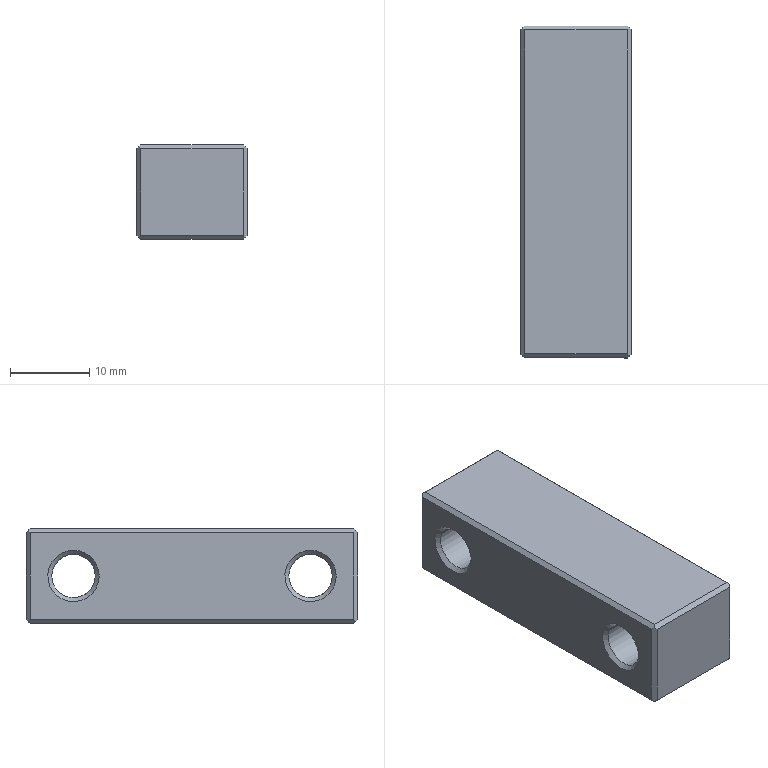CAM job | NX | 3+2 milling, drilling | part box 14 x 42 x 12 mm | stock box 20 x 47 x 15 mm
Tools:
number,name,description,diameter,corner_radius,flute_length,length,flutes
9,D10,平底铣刀-粗,10.0,0.0,35.0,75.0,2
10,D10-J,平底铣刀-精,10.0,0.0,35.0,75.0,2
1,D80R0.8飞刀,圆鼻刀-粗,80.0,0.8,50.0,75.0,2
2,D6倒角刀,倒角刀,6.0,0.0,3.0,25.0,2
24,ZT5.5,钻头,5.5,0.0,35.0,50.0,2
Operations:
program,operation,operation_type,tool,method,geometry_group,spindle_rpm,surface_speed,feed_per_tooth,feed_cut,feed_plunge,cut_length_mm,path_length_mm,cut_time_min,machine_time_min
A,顶面,FaceMilling,D80R0.8飞刀,侧刃精光-切深K-步距G,W-A,4000.0,1005.31,0.125,1000.0,100.0,136.0,172.0,0.136,0.1396
A,外形粗_2,VolumeBased25DMillingOperation,D10,METHOD,W-A,8000.0,251.327,0.3125,5000.0,80.0,2778.996,2831.996,0.5558,0.5611
A,打点-深0.8,Operation,D6倒角刀,NONE,W-A,8000.0,150.796,0.0312,500.0,90.0,3.6,78.217,0.0072,0.0147
A,通孔-5-6,Operation,ZT5.5,NONE,W-A,3000.0,51.836,0.025,150.0,90.0,37.305,145.626,0.2487,0.2595
A,铣倒角_1,PlanarMilling,D6倒角刀,METHOD,W-A,8000.0,150.796,0.0312,500.0,100.0,36.499,149.019,0.073,0.0842
A,底壁铣倒角_COPY,VolumeBased25DMillingOperation,D6倒角刀,爬面_倒角-切深0-步距G,W-A,6500.0,122.519,0.1154,1500.0,100.0,119.783,159.183,0.0799,0.0838
A,外形半精_2,VolumeBased25DMillingOperation,D10-J,METHOD,W-A,8000.0,251.327,0.0625,1000.0,100.0,143.202,211.202,0.1432,0.15